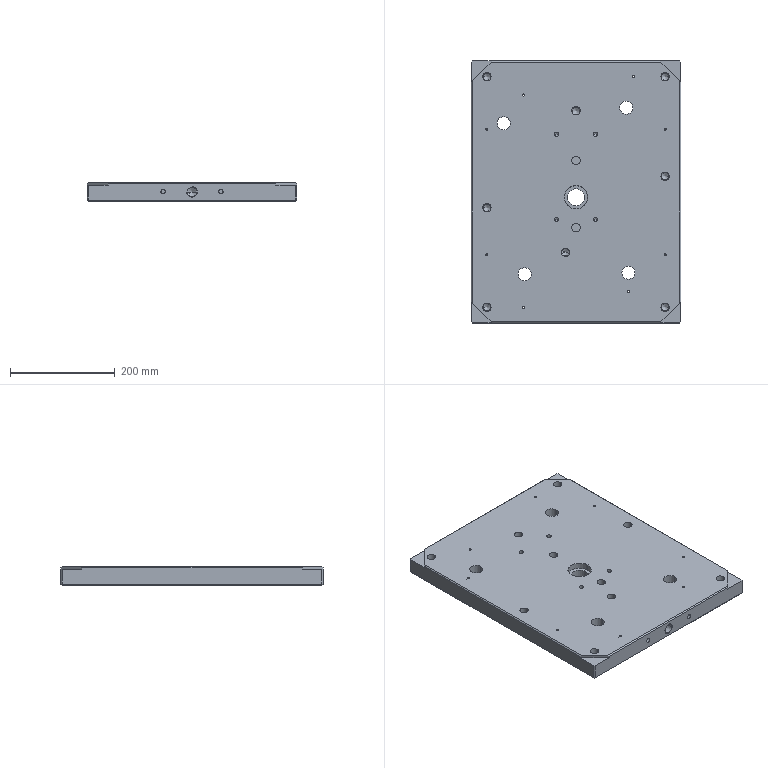Part | Creo | 1 solid | 513 faces | box 400 x 500 x 35 mm | volume 6668983 mm3 | plane 147 | other 138 | cylinder 132 | cone 96 | commonest cylinder face diameters 16 x40 13.9 x36 8 x26 8.5 x8 25 x8 17.4 x4